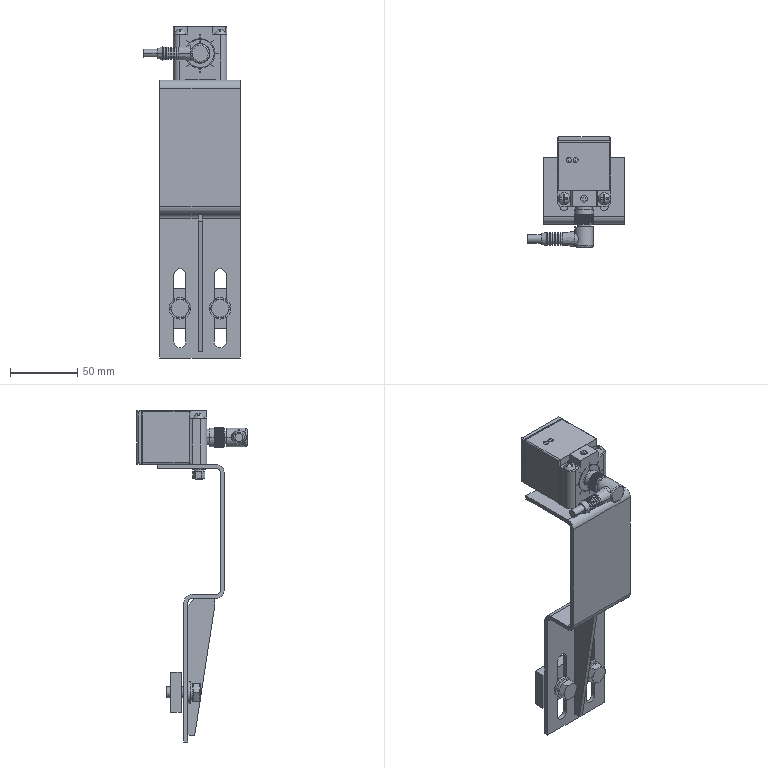Part | SolidWorks | 13 solids | 2100 faces | box 72 x 82 x 247.45 mm | volume 157229 mm3 | spline 1224 | cylinder 444 | plane 362 | cone 70 | commonest cylinder face diameters 14.5 x275 2 x14 6 x13 1 x10 5 x10 7.8 x10